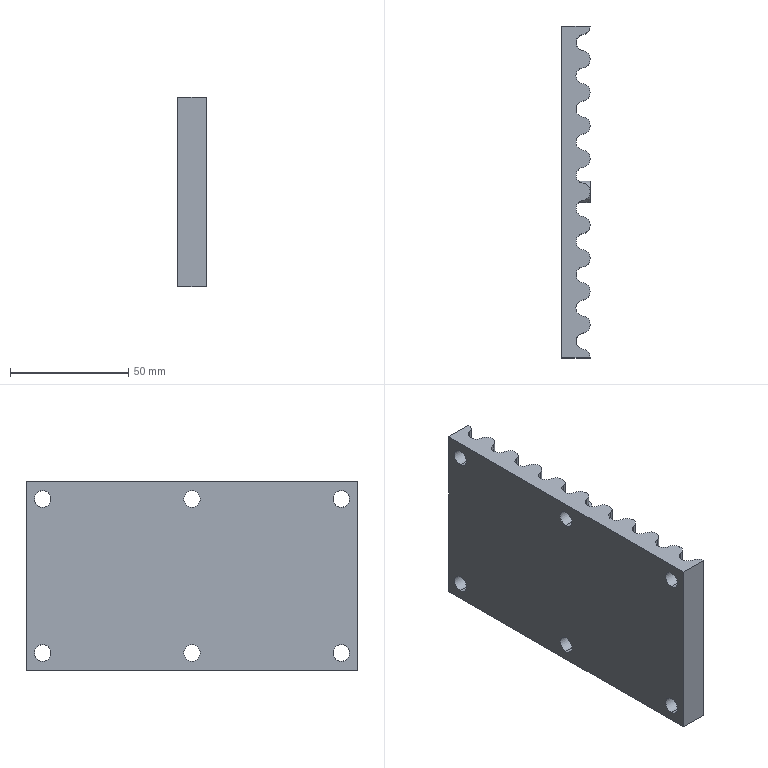Part | STEP file | LM-05-1155 modified_default | 1 solid | 86 faces | box 12 x 140 x 80 mm | volume 99342 mm3 | cylinder 66 | plane 16 | spline 4 | commonest cylinder face diameters 7 x62 9 x4